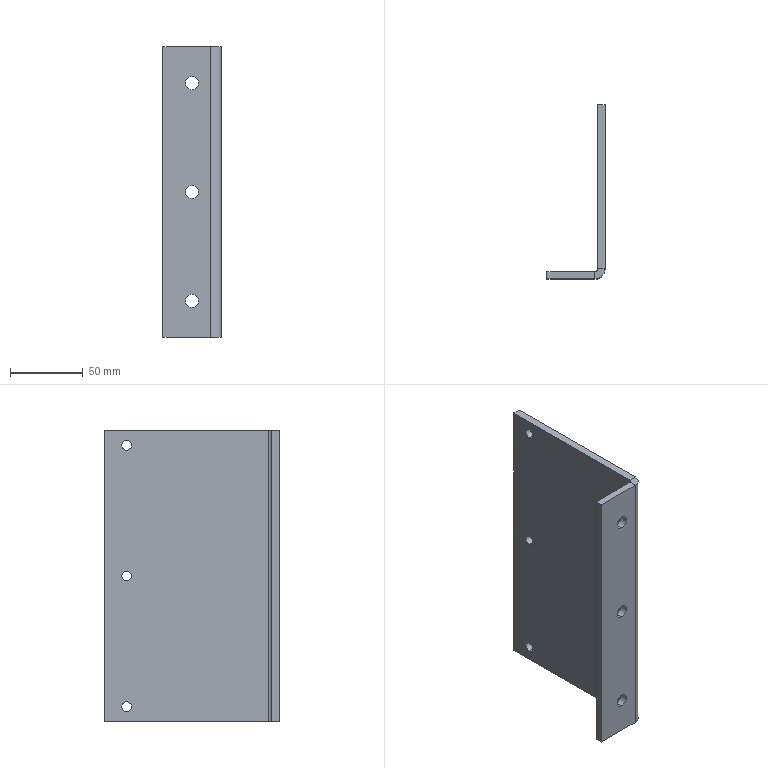Part | SolidWorks | features FlatPattern 1, HoleWzd 1, ICE 1, SMBaseFlange 1, SheetMetal 1 | 1 solid | 26 faces | box 40 x 120 x 200 mm | volume 151570 mm3 | cylinder 14 | plane 12 | commonest cylinder face diameters 6.8 x6 9 x6 4 x1 14 x1
STEP:
#1=CARTESIAN_POINT('',(40.,105.,186.6));
#2=VERTEX_POINT('',#1);
#3=CARTESIAN_POINT('',(40.,105.,193.4));
#4=VERTEX_POINT('',#3);
#5=CARTESIAN_POINT('',(40.,105.,190.));
#6=DIRECTION('',(-1.,0.,0.));
#7=DIRECTION('',(0.,0.,1.));
#8=AXIS2_PLACEMENT_3D('',#5,#6,#7);
#9=CIRCLE('',#8,3.4);
#10=EDGE_CURVE('',#2,#4,#9,.T.);
#11=ORIENTED_EDGE('',*,*,#10,.F.);
#12=CARTESIAN_POINT('',(35.,105.,186.6));
#13=VERTEX_POINT('',#12);
#14=CARTESIAN_POINT('',(35.,105.,186.6));
#15=DIRECTION('',(-1.,0.,0.));
#16=VECTOR('',#15,1000.);
#17=LINE('',#14,#16);
#18=EDGE_CURVE('',#2,#13,#17,.T.);
#19=ORIENTED_EDGE('',*,*,#18,.T.);
#20=CARTESIAN_POINT('',(35.,105.,193.4));
#21=VERTEX_POINT('',#20);
#22=CARTESIAN_POINT('',(35.,105.,190.));
#23=DIRECTION('',(-1.,0.,0.));
#24=DIRECTION('',(0.,0.,1.));
#25=AXIS2_PLACEMENT_3D('',#22,#23,#24);
#26=CIRCLE('',#25,3.4);
#27=EDGE_CURVE('',#13,#21,#26,.T.);
#28=ORIENTED_EDGE('',*,*,#27,.T.);
#29=CARTESIAN_POINT('',(35.,105.,193.4));
#30=DIRECTION('',(-1.,0.,0.));
#31=VECTOR('',#30,1000.);
#32=LINE('',#29,#31);
#33=EDGE_CURVE('',#4,#21,#32,.T.);
#34=ORIENTED_EDGE('',*,*,#33,.F.);
#35=EDGE_LOOP('',(#11,#19,#28,#34));
#36=FACE_OUTER_BOUND('',#35,.T.);
#37=CARTESIAN_POINT('',(35.,105.,190.));
#38=DIRECTION('',(-1.,0.,0.));
#39=DIRECTION('',(0.,0.,1.));
#40=AXIS2_PLACEMENT_3D('',#37,#38,#39);
#41=CYLINDRICAL_SURFACE('',#40,3.4);
#42=ADVANCED_FACE('',(#36),#41,.F.);
#43=CARTESIAN_POINT('',(40.,105.,96.6));
#44=VERTEX_POINT('',#43);
#45=CARTESIAN_POINT('',(40.,105.,103.4));
#46=VERTEX_POINT('',#45);
#47=CARTESIAN_POINT('',(40.,105.,100.));
#48=DIRECTION('',(-1.,0.,0.));
#49=DIRECTION('',(0.,0.,1.));
#50=AXIS2_PLACEMENT_3D('',#47,#48,#49);
#51=CIRCLE('',#50,3.4);
#52=EDGE_CURVE('',#44,#46,#51,.T.);
#53=ORIENTED_EDGE('',*,*,#52,.F.);
#54=CARTESIAN_POINT('',(35.,105.,96.6));
#55=VERTEX_POINT('',#54);
#56=CARTESIAN_POINT('',(35.,105.,96.6));
#57=DIRECTION('',(-1.,0.,0.));
#58=VECTOR('',#57,1000.);
#59=LINE('',#56,#58);
#60=EDGE_CURVE('',#44,#55,#59,.T.);
#61=ORIENTED_EDGE('',*,*,#60,.T.);
#62=CARTESIAN_POINT('',(35.,105.,103.4));
#63=VERTEX_POINT('',#62);
#64=CARTESIAN_POINT('',(35.,105.,100.));
#65=DIRECTION('',(-1.,0.,0.));
#66=DIRECTION('',(0.,0.,1.));
#67=AXIS2_PLACEMENT_3D('',#64,#65,#66);
#68=CIRCLE('',#67,3.4);
#69=EDGE_CURVE('',#55,#63,#68,.T.);
#70=ORIENTED_EDGE('',*,*,#69,.T.);
#71=CARTESIAN_POINT('',(35.,105.,103.4));
#72=DIRECTION('',(-1.,0.,0.));
#73=VECTOR('',#72,1000.);
#74=LINE('',#71,#73);
#75=EDGE_CURVE('',#46,#63,#74,.T.);
#76=ORIENTED_EDGE('',*,*,#75,.F.);
#77=EDGE_LOOP('',(#53,#61,#70,#76));
#78=FACE_OUTER_BOUND('',#77,.T.);
#79=CARTESIAN_POINT('',(35.,105.,100.));
#80=DIRECTION('',(-1.,0.,0.));
#81=DIRECTION('',(0.,0.,1.));
#82=AXIS2_PLACEMENT_3D('',#79,#80,#81);
#83=CYLINDRICAL_SURFACE('',#82,3.4);
#84=ADVANCED_FACE('',(#78),#83,.F.);
#85=CARTESIAN_POINT('',(40.,105.,6.6));
#86=VERTEX_POINT('',#85);
#87=CARTESIAN_POINT('',(40.,105.,13.4));
#88=VERTEX_POINT('',#87);
#89=CARTESIAN_POINT('',(40.,105.,10.));
#90=DIRECTION('',(-1.,0.,0.));
#91=DIRECTION('',(0.,0.,1.));
#92=AXIS2_PLACEMENT_3D('',#89,#90,#91);
#93=CIRCLE('',#92,3.4);
#94=EDGE_CURVE('',#86,#88,#93,.T.);
#95=ORIENTED_EDGE('',*,*,#94,.F.);
#96=CARTESIAN_POINT('',(35.,105.,6.6));
#97=VERTEX_POINT('',#96);
#98=CARTESIAN_POINT('',(35.,105.,6.6));
#99=DIRECTION('',(-1.,0.,0.));
#100=VECTOR('',#99,1000.);
#101=LINE('',#98,#100);
#102=EDGE_CURVE('',#86,#97,#101,.T.);
#103=ORIENTED_EDGE('',*,*,#102,.T.);
#104=CARTESIAN_POINT('',(35.,105.,13.4));
#105=VERTEX_POINT('',#104);
#106=CARTESIAN_POINT('',(35.,105.,10.));
#107=DIRECTION('',(-1.,0.,0.));
#108=DIRECTION('',(0.,0.,1.));
#109=AXIS2_PLACEMENT_3D('',#106,#107,#108);
#110=CIRCLE('',#109,3.4);
#111=EDGE_CURVE('',#97,#105,#110,.T.);
#112=ORIENTED_EDGE('',*,*,#111,.T.);
#113=CARTESIAN_POINT('',(35.,105.,13.4));
#114=DIRECTION('',(-1.,0.,0.));
#115=VECTOR('',#114,1000.);
#116=LINE('',#113,#115);
#117=EDGE_CURVE('',#88,#105,#116,.T.);
#118=ORIENTED_EDGE('',*,*,#117,.F.);
#119=EDGE_LOOP('',(#95,#103,#112,#118));
#120=FACE_OUTER_BOUND('',#119,.T.);
#121=CARTESIAN_POINT('',(35.,105.,10.));
#122=DIRECTION('',(-1.,0.,0.));
#123=DIRECTION('',(0.,0.,1.));
#124=AXIS2_PLACEMENT_3D('',#121,#122,#123);
#125=CYLINDRICAL_SURFACE('',#124,3.4);
#126=ADVANCED_FACE('',(#120),#125,.F.);
#127=CARTESIAN_POINT('',(20.,0.,170.5));
#128=VERTEX_POINT('',#127);
#129=CARTESIAN_POINT('',(20.,0.,179.5));
#130=VERTEX_POINT('',#129);
#131=CARTESIAN_POINT('',(20.,0.,175.));
#132=DIRECTION('',(0.,1.,0.));
#133=DIRECTION('',(0.,0.,1.));
#134=AXIS2_PLACEMENT_3D('',#131,#132,#133);
#135=CIRCLE('',#134,4.5);
#136=EDGE_CURVE('',#128,#130,#135,.T.);
#137=ORIENTED_EDGE('',*,*,#136,.F.);
#138=CARTESIAN_POINT('',(20.,5.,170.5));
#139=VERTEX_POINT('',#138);
#140=CARTESIAN_POINT('',(20.,-5.,170.5));
#141=DIRECTION('',(0.,1.,0.));
#142=VECTOR('',#141,1000.);
#143=LINE('',#140,#142);
#144=EDGE_CURVE('',#128,#139,#143,.T.);
#145=ORIENTED_EDGE('',*,*,#144,.T.);
#146=CARTESIAN_POINT('',(20.,5.,179.5));
#147=VERTEX_POINT('',#146);
#148=CARTESIAN_POINT('',(20.,5.,175.));
#149=DIRECTION('',(0.,1.,0.));
#150=DIRECTION('',(0.,0.,1.));
#151=AXIS2_PLACEMENT_3D('',#148,#149,#150);
#152=CIRCLE('',#151,4.5);
#153=EDGE_CURVE('',#139,#147,#152,.T.);
#154=ORIENTED_EDGE('',*,*,#153,.T.);
#155=CARTESIAN_POINT('',(20.,-5.,179.5));
#156=DIRECTION('',(0.,1.,0.));
#157=VECTOR('',#156,1000.);
#158=LINE('',#155,#157);
#159=EDGE_CURVE('',#130,#147,#158,.T.);
#160=ORIENTED_EDGE('',*,*,#159,.F.);
#161=EDGE_LOOP('',(#137,#145,#154,#160));
#162=FACE_OUTER_BOUND('',#161,.T.);
#163=CARTESIAN_POINT('',(20.,-5.,175.));
#164=DIRECTION('',(0.,1.,0.));
#165=DIRECTION('',(0.,0.,1.));
#166=AXIS2_PLACEMENT_3D('',#163,#164,#165);
#167=CYLINDRICAL_SURFACE('',#166,4.5);
#168=ADVANCED_FACE('',(#162),#167,.F.);
#169=CARTESIAN_POINT('',(20.,0.,95.5));
#170=VERTEX_POINT('',#169);
#171=CARTESIAN_POINT('',(20.,0.,104.5));
#172=VERTEX_POINT('',#171);
#173=CARTESIAN_POINT('',(20.,0.,100.));
#174=DIRECTION('',(0.,1.,0.));
#175=DIRECTION('',(0.,0.,1.));
#176=AXIS2_PLACEMENT_3D('',#173,#174,#175);
#177=CIRCLE('',#176,4.5);
#178=EDGE_CURVE('',#170,#172,#177,.T.);
#179=ORIENTED_EDGE('',*,*,#178,.F.);
#180=CARTESIAN_POINT('',(20.,5.,95.5));
#181=VERTEX_POINT('',#180);
#182=CARTESIAN_POINT('',(20.,-5.,95.5));
#183=DIRECTION('',(0.,1.,0.));
#184=VECTOR('',#183,1000.);
#185=LINE('',#182,#184);
#186=EDGE_CURVE('',#170,#181,#185,.T.);
#187=ORIENTED_EDGE('',*,*,#186,.T.);
#188=CARTESIAN_POINT('',(20.,5.,104.5));
#189=VERTEX_POINT('',#188);
#190=CARTESIAN_POINT('',(20.,5.,100.));
#191=DIRECTION('',(0.,1.,0.));
#192=DIRECTION('',(0.,0.,1.));
#193=AXIS2_PLACEMENT_3D('',#190,#191,#192);
#194=CIRCLE('',#193,4.5);
#195=EDGE_CURVE('',#181,#189,#194,.T.);
#196=ORIENTED_EDGE('',*,*,#195,.T.);
#197=CARTESIAN_POINT('',(20.,-5.,104.5));
#198=DIRECTION('',(0.,1.,0.));
#199=VECTOR('',#198,1000.);
#200=LINE('',#197,#199);
#201=EDGE_CURVE('',#172,#189,#200,.T.);
#202=ORIENTED_EDGE('',*,*,#201,.F.);
#203=EDGE_LOOP('',(#179,#187,#196,#202));
#204=FACE_OUTER_BOUND('',#203,.T.);
#205=CARTESIAN_POINT('',(20.,-5.,100.));
#206=DIRECTION('',(0.,1.,0.));
#207=DIRECTION('',(0.,0.,1.));
#208=AXIS2_PLACEMENT_3D('',#205,#206,#207);
#209=CYLINDRICAL_SURFACE('',#208,4.5);
#210=ADVANCED_FACE('',(#204),#209,.F.);
#211=CARTESIAN_POINT('',(20.,0.,20.5));
#212=VERTEX_POINT('',#211);
#213=CARTESIAN_POINT('',(20.,0.,29.5));
#214=VERTEX_POINT('',#213);
#215=CARTESIAN_POINT('',(20.,0.,25.));
#216=DIRECTION('',(0.,1.,0.));
#217=DIRECTION('',(0.,0.,1.));
#218=AXIS2_PLACEMENT_3D('',#215,#216,#217);
#219=CIRCLE('',#218,4.5);
#220=EDGE_CURVE('',#212,#214,#219,.T.);
#221=ORIENTED_EDGE('',*,*,#220,.F.);
#222=CARTESIAN_POINT('',(20.,5.,20.5));
#223=VERTEX_POINT('',#222);
#224=CARTESIAN_POINT('',(20.,-5.,20.5));
#225=DIRECTION('',(0.,1.,0.));
#226=VECTOR('',#225,1000.);
#227=LINE('',#224,#226);
#228=EDGE_CURVE('',#212,#223,#227,.T.);
#229=ORIENTED_EDGE('',*,*,#228,.T.);
#230=CARTESIAN_POINT('',(20.,5.,29.5));
#231=VERTEX_POINT('',#230);
#232=CARTESIAN_POINT('',(20.,5.,25.));
#233=DIRECTION('',(0.,1.,0.));
#234=DIRECTION('',(0.,0.,1.));
#235=AXIS2_PLACEMENT_3D('',#232,#233,#234);
#236=CIRCLE('',#235,4.5);
#237=EDGE_CURVE('',#223,#231,#236,.T.);
#238=ORIENTED_EDGE('',*,*,#237,.T.);
#239=CARTESIAN_POINT('',(20.,-5.,29.5));
#240=DIRECTION('',(0.,1.,0.));
#241=VECTOR('',#240,1000.);
#242=LINE('',#239,#241);
#243=EDGE_CURVE('',#214,#231,#242,.T.);
#244=ORIENTED_EDGE('',*,*,#243,.F.);
#245=EDGE_LOOP('',(#221,#229,#238,#244));
#246=FACE_OUTER_BOUND('',#245,.T.);
#247=CARTESIAN_POINT('',(20.,-5.,25.));
#248=DIRECTION('',(0.,1.,0.));
#249=DIRECTION('',(0.,0.,1.));
#250=AXIS2_PLACEMENT_3D('',#247,#248,#249);
#251=CYLINDRICAL_SURFACE('',#250,4.5);
#252=ADVANCED_FACE('',(#246),#251,.F.);
#253=CARTESIAN_POINT('',(33.,0.,200.));
#254=VERTEX_POINT('',#253);
#255=CARTESIAN_POINT('',(33.,5.,200.));
#256=VERTEX_POINT('',#255);
#257=CARTESIAN_POINT('',(33.,0.,200.));
#258=DIRECTION('',(0.,1.,0.));
#259=VECTOR('',#258,1000.);
#260=LINE('',#257,#259);
#261=EDGE_CURVE('',#254,#256,#260,.T.);
#262=ORIENTED_EDGE('',*,*,#261,.F.);
#263=CARTESIAN_POINT('',(40.,7.,200.));
#264=VERTEX_POINT('',#263);
#265=CARTESIAN_POINT('',(33.,7.,200.));
#266=DIRECTION('',(0.,0.,1.));
#267=DIRECTION('',(-1.,0.,0.));
#268=AXIS2_PLACEMENT_3D('',#265,#266,#267);
#269=CIRCLE('',#268,7.);
#270=EDGE_CURVE('',#254,#264,#269,.T.);
#271=ORIENTED_EDGE('',*,*,#270,.T.);
#272=CARTESIAN_POINT('',(35.,7.,200.));
#273=VERTEX_POINT('',#272);
#274=CARTESIAN_POINT('',(35.,7.,200.));
#275=DIRECTION('',(1.,0.,0.));
#276=VECTOR('',#275,1000.);
#277=LINE('',#274,#276);
#278=EDGE_CURVE('',#273,#264,#277,.T.);
#279=ORIENTED_EDGE('',*,*,#278,.F.);
#280=CARTESIAN_POINT('',(33.,7.,200.));
#281=DIRECTION('',(0.,0.,1.));
#282=DIRECTION('',(1.,0.,0.));
#283=AXIS2_PLACEMENT_3D('',#280,#281,#282);
#284=CIRCLE('',#283,2.);
#285=EDGE_CURVE('',#256,#273,#284,.T.);
#286=ORIENTED_EDGE('',*,*,#285,.F.);
#287=EDGE_LOOP('',(#262,#271,#279,#286));
#288=FACE_OUTER_BOUND('',#287,.T.);
#289=CARTESIAN_POINT('',(33.,0.,200.));
#290=DIRECTION('',(0.,0.,1.));
#291=DIRECTION('',(1.,0.,0.));
#292=AXIS2_PLACEMENT_3D('',#289,#290,#291);
#293=PLANE('',#292);
#294=ADVANCED_FACE('',(#288),#293,.T.);
#295=CARTESIAN_POINT('',(0.,0.,200.));
#296=VERTEX_POINT('',#295);
#297=CARTESIAN_POINT('',(0.,0.,200.));
#298=DIRECTION('',(1.,0.,0.));
#299=VECTOR('',#298,1000.);
#300=LINE('',#297,#299);
#301=EDGE_CURVE('',#296,#254,#300,.T.);
#302=ORIENTED_EDGE('',*,*,#301,.T.);
#303=ORIENTED_EDGE('',*,*,#261,.T.);
#304=CARTESIAN_POINT('',(0.,5.,200.));
#305=VERTEX_POINT('',#304);
#306=CARTESIAN_POINT('',(0.,5.,200.));
#307=DIRECTION('',(1.,0.,0.));
#308=VECTOR('',#307,1000.);
#309=LINE('',#306,#308);
#310=EDGE_CURVE('',#305,#256,#309,.T.);
#311=ORIENTED_EDGE('',*,*,#310,.F.);
#312=CARTESIAN_POINT('',(0.,0.,200.));
#313=DIRECTION('',(0.,1.,0.));
#314=VECTOR('',#313,1000.);
#315=LINE('',#312,#314);
#316=EDGE_CURVE('',#296,#305,#315,.T.);
#317=ORIENTED_EDGE('',*,*,#316,.F.);
#318=EDGE_LOOP('',(#302,#303,#311,#317));
#319=FACE_OUTER_BOUND('',#318,.T.);
#320=CARTESIAN_POINT('',(35.,7.,200.));
#321=DIRECTION('',(0.,0.,1.));
#322=DIRECTION('',(1.,0.,0.));
#323=AXIS2_PLACEMENT_3D('',#320,#321,#322);
#324=PLANE('',#323);
#325=ADVANCED_FACE('',(#319),#324,.T.);
#326=CARTESIAN_POINT('',(40.,7.,0.));
#327=VERTEX_POINT('',#326);
#328=CARTESIAN_POINT('',(35.,7.,0.));
#329=VERTEX_POINT('',#328);
#330=CARTESIAN_POINT('',(40.,7.,0.));
#331=DIRECTION('',(-1.,0.,0.));
#332=VECTOR('',#331,1000.);
#333=LINE('',#330,#332);
#334=EDGE_CURVE('',#327,#329,#333,.T.);
#335=ORIENTED_EDGE('',*,*,#334,.F.);
#336=CARTESIAN_POINT('',(33.,0.,0.));
#337=VERTEX_POINT('',#336);
#338=CARTESIAN_POINT('',(33.,7.,0.));
#339=DIRECTION('',(0.,0.,1.));
#340=DIRECTION('',(-1.,0.,0.));
#341=AXIS2_PLACEMENT_3D('',#338,#339,#340);
#342=CIRCLE('',#341,7.);
#343=EDGE_CURVE('',#337,#327,#342,.T.);
#344=ORIENTED_EDGE('',*,*,#343,.F.);
#345=CARTESIAN_POINT('',(33.,5.,0.));
#346=VERTEX_POINT('',#345);
#347=CARTESIAN_POINT('',(33.,5.,0.));
#348=DIRECTION('',(0.,-1.,0.));
#349=VECTOR('',#348,1000.);
#350=LINE('',#347,#349);
#351=EDGE_CURVE('',#346,#337,#350,.T.);
#352=ORIENTED_EDGE('',*,*,#351,.F.);
#353=CARTESIAN_POINT('',(33.,7.,0.));
#354=DIRECTION('',(0.,0.,1.));
#355=DIRECTION('',(1.,0.,0.));
#356=AXIS2_PLACEMENT_3D('',#353,#354,#355);
#357=CIRCLE('',#356,2.);
#358=EDGE_CURVE('',#346,#329,#357,.T.);
#359=ORIENTED_EDGE('',*,*,#358,.T.);
#360=EDGE_LOOP('',(#335,#344,#352,#359));
#361=FACE_OUTER_BOUND('',#360,.T.);
#362=CARTESIAN_POINT('',(40.,7.,0.));
#363=DIRECTION('',(0.,0.,-1.));
#364=DIRECTION('',(-1.,0.,0.));
#365=AXIS2_PLACEMENT_3D('',#362,#363,#364);
#366=PLANE('',#365);
#367=ADVANCED_FACE('',(#361),#366,.T.);
#368=CARTESIAN_POINT('',(40.,120.,0.));
#369=VERTEX_POINT('',#368);
#370=CARTESIAN_POINT('',(40.,0.,0.));
#371=DIRECTION('',(0.,1.,0.));
#372=VECTOR('',#371,1000.);
#373=LINE('',#370,#372);
#374=EDGE_CURVE('',#327,#369,#373,.T.);
#375=ORIENTED_EDGE('',*,*,#374,.F.);
#376=ORIENTED_EDGE('',*,*,#334,.T.);
#377=CARTESIAN_POINT('',(35.,120.,0.));
#378=VERTEX_POINT('',#377);
#379=CARTESIAN_POINT('',(35.,0.,0.));
#380=DIRECTION('',(0.,1.,0.));
#381=VECTOR('',#380,1000.);
#382=LINE('',#379,#381);
#383=EDGE_CURVE('',#329,#378,#382,.T.);
#384=ORIENTED_EDGE('',*,*,#383,.T.);
#385=CARTESIAN_POINT('',(35.,120.,0.));
#386=DIRECTION('',(1.,0.,0.));
#387=VECTOR('',#386,1000.);
#388=LINE('',#385,#387);
#389=EDGE_CURVE('',#378,#369,#388,.T.);
#390=ORIENTED_EDGE('',*,*,#389,.T.);
#391=EDGE_LOOP('',(#375,#376,#384,#390));
#392=FACE_OUTER_BOUND('',#391,.T.);
#393=CARTESIAN_POINT('',(33.,5.,0.));
#394=DIRECTION('',(0.,0.,-1.));
#395=DIRECTION('',(-1.,0.,0.));
#396=AXIS2_PLACEMENT_3D('',#393,#394,#395);
#397=PLANE('',#396);
#398=ADVANCED_FACE('',(#392),#397,.T.);
#399=CARTESIAN_POINT('',(40.,105.,190.));
#400=DIRECTION('',(-1.,0.,0.));
#401=DIRECTION('',(0.,0.,1.));
#402=AXIS2_PLACEMENT_3D('',#399,#400,#401);
#403=CIRCLE('',#402,3.4);
#404=EDGE_CURVE('',#4,#2,#403,.T.);
#405=ORIENTED_EDGE('',*,*,#404,.T.);
#406=ORIENTED_EDGE('',*,*,#10,.T.);
#407=EDGE_LOOP('',(#405,#406));
#408=FACE_BOUND('',#407,.T.);
#409=CARTESIAN_POINT('',(40.,105.,100.));
#410=DIRECTION('',(-1.,0.,0.));
#411=DIRECTION('',(0.,0.,1.));
#412=AXIS2_PLACEMENT_3D('',#409,#410,#411);
#413=CIRCLE('',#412,3.4);
#414=EDGE_CURVE('',#46,#44,#413,.T.);
#415=ORIENTED_EDGE('',*,*,#414,.T.);
#416=ORIENTED_EDGE('',*,*,#52,.T.);
#417=EDGE_LOOP('',(#415,#416));
#418=FACE_BOUND('',#417,.T.);
#419=CARTESIAN_POINT('',(40.,105.,10.));
#420=DIRECTION('',(-1.,0.,0.));
#421=DIRECTION('',(0.,0.,1.));
#422=AXIS2_PLACEMENT_3D('',#419,#420,#421);
#423=CIRCLE('',#422,3.4);
#424=EDGE_CURVE('',#88,#86,#423,.T.);
#425=ORIENTED_EDGE('',*,*,#424,.T.);
#426=ORIENTED_EDGE('',*,*,#94,.T.);
#427=EDGE_LOOP('',(#425,#426));
#428=FACE_BOUND('',#427,.T.);
#429=ORIENTED_EDGE('',*,*,#374,.T.);
#430=CARTESIAN_POINT('',(40.,120.,200.));
#431=VERTEX_POINT('',#430);
#432=CARTESIAN_POINT('',(40.,120.,200.));
#433=DIRECTION('',(0.,0.,-1.));
#434=VECTOR('',#433,1000.);
#435=LINE('',#432,#434);
#436=EDGE_CURVE('',#431,#369,#435,.T.);
#437=ORIENTED_EDGE('',*,*,#436,.F.);
#438=CARTESIAN_POINT('',(40.,0.,200.));
#439=DIRECTION('',(0.,1.,0.));
#440=VECTOR('',#439,1000.);
#441=LINE('',#438,#440);
#442=EDGE_CURVE('',#264,#431,#441,.T.);
#443=ORIENTED_EDGE('',*,*,#442,.F.);
#444=CARTESIAN_POINT('',(40.,7.,200.));
#445=DIRECTION('',(0.,0.,-1.));
#446=VECTOR('',#445,1000.);
#447=LINE('',#444,#446);
#448=EDGE_CURVE('',#264,#327,#447,.T.);
#449=ORIENTED_EDGE('',*,*,#448,.T.);
#450=EDGE_LOOP('',(#429,#437,#443,#449));
#451=FACE_OUTER_BOUND('',#450,.T.);
#452=CARTESIAN_POINT('',(40.,0.,200.));
#453=DIRECTION('',(-1.,0.,0.));
#454=DIRECTION('',(0.,0.,1.));
#455=AXIS2_PLACEMENT_3D('',#452,#453,#454);
#456=PLANE('',#455);
#457=ADVANCED_FACE('',(#408,#418,#428,#451),#456,.F.);
#458=ORIENTED_EDGE('',*,*,#389,.F.);
#459=CARTESIAN_POINT('',(35.,120.,200.));
#460=VERTEX_POINT('',#459);
#461=CARTESIAN_POINT('',(35.,120.,200.));
#462=DIRECTION('',(0.,0.,-1.));
#463=VECTOR('',#462,1000.);
#464=LINE('',#461,#463);
#465=EDGE_CURVE('',#460,#378,#464,.T.);
#466=ORIENTED_EDGE('',*,*,#465,.F.);
#467=CARTESIAN_POINT('',(35.,120.,200.));
#468=DIRECTION('',(1.,0.,0.));
#469=VECTOR('',#468,1000.);
#470=LINE('',#467,#469);
#471=EDGE_CURVE('',#460,#431,#470,.T.);
#472=ORIENTED_EDGE('',*,*,#471,.T.);
#473=ORIENTED_EDGE('',*,*,#436,.T.);
#474=EDGE_LOOP('',(#458,#466,#472,#473));
#475=FACE_OUTER_BOUND('',#474,.T.);
#476=CARTESIAN_POINT('',(35.,120.,200.));
#477=DIRECTION('',(0.,1.,0.));
#478=DIRECTION('',(0.,0.,1.));
#479=AXIS2_PLACEMENT_3D('',#476,#477,#478);
#480=PLANE('',#479);
#481=ADVANCED_FACE('',(#475),#480,.T.);
#482=CARTESIAN_POINT('',(35.,105.,190.));
#483=DIRECTION('',(-1.,0.,0.));
#484=DIRECTION('',(0.,0.,1.));
#485=AXIS2_PLACEMENT_3D('',#482,#483,#484);
#486=CIRCLE('',#485,3.4);
#487=EDGE_CURVE('',#21,#13,#486,.T.);
#488=ORIENTED_EDGE('',*,*,#487,.F.);
#489=ORIENTED_EDGE('',*,*,#27,.F.);
#490=EDGE_LOOP('',(#488,#489));
#491=FACE_BOUND('',#490,.T.);
#492=CARTESIAN_POINT('',(35.,105.,100.));
#493=DIRECTION('',(-1.,0.,0.));
#494=DIRECTION('',(0.,0.,1.));
#495=AXIS2_PLACEMENT_3D('',#492,#493,#494);
#496=CIRCLE('',#495,3.4);
#497=EDGE_CURVE('',#63,#55,#496,.T.);
#498=ORIENTED_EDGE('',*,*,#497,.F.);
#499=ORIENTED_EDGE('',*,*,#69,.F.);
#500=EDGE_LOOP('',(#498,#499));
#501=FACE_BOUND('',#500,.T.);
#502=CARTESIAN_POINT('',(35.,105.,10.));
#503=DIRECTION('',(-1.,0.,0.));
#504=DIRECTION('',(0.,0.,1.));
#505=AXIS2_PLACEMENT_3D('',#502,#503,#504);
#506=CIRCLE('',#505,3.4);
#507=EDGE_CURVE('',#105,#97,#506,.T.);
#508=ORIENTED_EDGE('',*,*,#507,.F.);
#509=ORIENTED_EDGE('',*,*,#111,.F.);
#510=EDGE_LOOP('',(#508,#509));
#511=FACE_BOUND('',#510,.T.);
#512=ORIENTED_EDGE('',*,*,#383,.F.);
#513=CARTESIAN_POINT('',(35.,7.,200.));
#514=DIRECTION('',(0.,0.,-1.));
#515=VECTOR('',#514,1000.);
#516=LINE('',#513,#515);
#517=EDGE_CURVE('',#273,#329,#516,.T.);
#518=ORIENTED_EDGE('',*,*,#517,.F.);
#519=CARTESIAN_POINT('',(35.,0.,200.));
#520=DIRECTION('',(0.,1.,0.));
#521=VECTOR('',#520,1000.);
#522=LINE('',#519,#521);
#523=EDGE_CURVE('',#273,#460,#522,.T.);
#524=ORIENTED_EDGE('',*,*,#523,.T.);
#525=ORIENTED_EDGE('',*,*,#465,.T.);
#526=EDGE_LOOP('',(#512,#518,#524,#525));
#527=FACE_OUTER_BOUND('',#526,.T.);
#528=CARTESIAN_POINT('',(35.,0.,200.));
#529=DIRECTION('',(-1.,0.,0.));
#530=DIRECTION('',(0.,0.,1.));
#531=AXIS2_PLACEMENT_3D('',#528,#529,#530);
#532=PLANE('',#531);
#533=ADVANCED_FACE('',(#491,#501,#511,#527),#532,.T.);
#534=ORIENTED_EDGE('',*,*,#358,.F.);
#535=CARTESIAN_POINT('',(33.,5.,200.));
#536=DIRECTION('',(0.,0.,-1.));
#537=VECTOR('',#536,1000.);
#538=LINE('',#535,#537);
#539=EDGE_CURVE('',#256,#346,#538,.T.);
#540=ORIENTED_EDGE('',*,*,#539,.F.);
#541=ORIENTED_EDGE('',*,*,#285,.T.);
#542=ORIENTED_EDGE('',*,*,#517,.T.);
#543=EDGE_LOOP('',(#534,#540,#541,#542));
#544=FACE_OUTER_BOUND('',#543,.T.);
#545=CARTESIAN_POINT('',(33.,7.,200.));
#546=DIRECTION('',(0.,0.,-1.));
#547=DIRECTION('',(-1.,0.,0.));
#548=AXIS2_PLACEMENT_3D('',#545,#546,#547);
#549=CYLINDRICAL_SURFACE('',#548,2.);
#550=ADVANCED_FACE('',(#544),#549,.F.);
#551=CARTESIAN_POINT('',(20.,5.,175.));
#552=DIRECTION('',(0.,1.,0.));
#553=DIRECTION('',(0.,0.,1.));
#554=AXIS2_PLACEMENT_3D('',#551,#552,#553);
#555=CIRCLE('',#554,4.5);
#556=EDGE_CURVE('',#147,#139,#555,.T.);
#557=ORIENTED_EDGE('',*,*,#556,.F.);
#558=ORIENTED_EDGE('',*,*,#153,.F.);
#559=EDGE_LOOP('',(#557,#558));
#560=FACE_BOUND('',#559,.T.);
#561=CARTESIAN_POINT('',(20.,5.,100.));
#562=DIRECTION('',(0.,1.,0.));
#563=DIRECTION('',(0.,0.,1.));
#564=AXIS2_PLACEMENT_3D('',#561,#562,#563);
#565=CIRCLE('',#564,4.5);
#566=EDGE_CURVE('',#189,#181,#565,.T.);
#567=ORIENTED_EDGE('',*,*,#566,.F.);
#568=ORIENTED_EDGE('',*,*,#195,.F.);
#569=EDGE_LOOP('',(#567,#568));
#570=FACE_BOUND('',#569,.T.);
#571=CARTESIAN_POINT('',(20.,5.,25.));
#572=DIRECTION('',(0.,1.,0.));
#573=DIRECTION('',(0.,0.,1.));
#574=AXIS2_PLACEMENT_3D('',#571,#572,#573);
#575=CIRCLE('',#574,4.5);
#576=EDGE_CURVE('',#231,#223,#575,.T.);
#577=ORIENTED_EDGE('',*,*,#576,.F.);
#578=ORIENTED_EDGE('',*,*,#237,.F.);
#579=EDGE_LOOP('',(#577,#578));
#580=FACE_BOUND('',#579,.T.);
#581=CARTESIAN_POINT('',(0.,5.,0.));
#582=VERTEX_POINT('',#581);
#583=CARTESIAN_POINT('',(0.,5.,0.));
#584=DIRECTION('',(1.,0.,0.));
#585=VECTOR('',#584,1000.);
#586=LINE('',#583,#585);
#587=EDGE_CURVE('',#582,#346,#586,.T.);
#588=ORIENTED_EDGE('',*,*,#587,.F.);
#589=CARTESIAN_POINT('',(0.,5.,200.));
#590=DIRECTION('',(0.,0.,-1.));
#591=VECTOR('',#590,1000.);
#592=LINE('',#589,#591);
#593=EDGE_CURVE('',#305,#582,#592,.T.);
#594=ORIENTED_EDGE('',*,*,#593,.F.);
#595=ORIENTED_EDGE('',*,*,#310,.T.);
#596=ORIENTED_EDGE('',*,*,#539,.T.);
#597=EDGE_LOOP('',(#588,#594,#595,#596));
#598=FACE_OUTER_BOUND('',#597,.T.);
#599=CARTESIAN_POINT('',(0.,5.,200.));
#600=DIRECTION('',(0.,1.,0.));
#601=DIRECTION('',(0.,0.,1.));
#602=AXIS2_PLACEMENT_3D('',#599,#600,#601);
#603=PLANE('',#602);
#604=ADVANCED_FACE('',(#560,#570,#580,#598),#603,.T.);
#605=CARTESIAN_POINT('',(0.,0.,0.));
#606=VERTEX_POINT('',#605);
#607=CARTESIAN_POINT('',(0.,0.,0.));
#608=DIRECTION('',(0.,1.,0.));
#609=VECTOR('',#608,1000.);
#610=LINE('',#607,#609);
#611=EDGE_CURVE('',#606,#582,#610,.T.);
#612=ORIENTED_EDGE('',*,*,#611,.F.);
#613=CARTESIAN_POINT('',(0.,0.,200.));
#614=DIRECTION('',(0.,0.,-1.));
#615=VECTOR('',#614,1000.);
#616=LINE('',#613,#615);
#617=EDGE_CURVE('',#296,#606,#616,.T.);
#618=ORIENTED_EDGE('',*,*,#617,.F.);
#619=ORIENTED_EDGE('',*,*,#316,.T.);
#620=ORIENTED_EDGE('',*,*,#593,.T.);
#621=EDGE_LOOP('',(#612,#618,#619,#620));
#622=FACE_OUTER_BOUND('',#621,.T.);
#623=CARTESIAN_POINT('',(0.,0.,200.));
#624=DIRECTION('',(-1.,0.,0.));
#625=DIRECTION('',(0.,0.,1.));
#626=AXIS2_PLACEMENT_3D('',#623,#624,#625);
#627=PLANE('',#626);
#628=ADVANCED_FACE('',(#622),#627,.T.);
#629=CARTESIAN_POINT('',(20.,0.,175.));
#630=DIRECTION('',(0.,1.,0.));
#631=DIRECTION('',(0.,0.,1.));
#632=AXIS2_PLACEMENT_3D('',#629,#630,#631);
#633=CIRCLE('',#632,4.5);
#634=EDGE_CURVE('',#130,#128,#633,.T.);
#635=ORIENTED_EDGE('',*,*,#634,.T.);
#636=ORIENTED_EDGE('',*,*,#136,.T.);
#637=EDGE_LOOP('',(#635,#636));
#638=FACE_BOUND('',#637,.T.);
#639=CARTESIAN_POINT('',(20.,0.,100.));
#640=DIRECTION('',(0.,1.,0.));
#641=DIRECTION('',(0.,0.,1.));
#642=AXIS2_PLACEMENT_3D('',#639,#640,#641);
#643=CIRCLE('',#642,4.5);
#644=EDGE_CURVE('',#172,#170,#643,.T.);
#645=ORIENTED_EDGE('',*,*,#644,.T.);
#646=ORIENTED_EDGE('',*,*,#178,.T.);
#647=EDGE_LOOP('',(#645,#646));
#648=FACE_BOUND('',#647,.T.);
#649=CARTESIAN_POINT('',(20.,0.,25.));
#650=DIRECTION('',(0.,1.,0.));
#651=DIRECTION('',(0.,0.,1.));
#652=AXIS2_PLACEMENT_3D('',#649,#650,#651);
#653=CIRCLE('',#652,4.5);
#654=EDGE_CURVE('',#214,#212,#653,.T.);
#655=ORIENTED_EDGE('',*,*,#654,.T.);
#656=ORIENTED_EDGE('',*,*,#220,.T.);
#657=EDGE_LOOP('',(#655,#656));
#658=FACE_BOUND('',#657,.T.);
#659=CARTESIAN_POINT('',(0.,0.,0.));
#660=DIRECTION('',(1.,0.,0.));
#661=VECTOR('',#660,1000.);
#662=LINE('',#659,#661);
#663=EDGE_CURVE('',#606,#337,#662,.T.);
#664=ORIENTED_EDGE('',*,*,#663,.T.);
#665=CARTESIAN_POINT('',(33.,0.,200.));
#666=DIRECTION('',(0.,0.,-1.));
#667=VECTOR('',#666,1000.);
#668=LINE('',#665,#667);
#669=EDGE_CURVE('',#254,#337,#668,.T.);
#670=ORIENTED_EDGE('',*,*,#669,.F.);
#671=ORIENTED_EDGE('',*,*,#301,.F.);
#672=ORIENTED_EDGE('',*,*,#617,.T.);
#673=EDGE_LOOP('',(#664,#670,#671,#672));
#674=FACE_OUTER_BOUND('',#673,.T.);
#675=CARTESIAN_POINT('',(0.,0.,200.));
#676=DIRECTION('',(0.,1.,0.));
#677=DIRECTION('',(0.,0.,1.));
#678=AXIS2_PLACEMENT_3D('',#675,#676,#677);
#679=PLANE('',#678);
#680=ADVANCED_FACE('',(#638,#648,#658,#674),#679,.F.);
#681=ORIENTED_EDGE('',*,*,#343,.T.);
#682=ORIENTED_EDGE('',*,*,#448,.F.);
#683=ORIENTED_EDGE('',*,*,#270,.F.);
#684=ORIENTED_EDGE('',*,*,#669,.T.);
#685=EDGE_LOOP('',(#681,#682,#683,#684));
#686=FACE_OUTER_BOUND('',#685,.T.);
#687=CARTESIAN_POINT('',(33.,7.,200.));
#688=DIRECTION('',(0.,0.,-1.));
#689=DIRECTION('',(-1.,0.,0.));
#690=AXIS2_PLACEMENT_3D('',#687,#688,#689);
#691=CYLINDRICAL_SURFACE('',#690,7.);
#692=ADVANCED_FACE('',(#686),#691,.T.);
#693=ORIENTED_EDGE('',*,*,#442,.T.);
#694=ORIENTED_EDGE('',*,*,#471,.F.);
#695=ORIENTED_EDGE('',*,*,#523,.F.);
#696=ORIENTED_EDGE('',*,*,#278,.T.);
#697=EDGE_LOOP('',(#693,#694,#695,#696));
#698=FACE_OUTER_BOUND('',#697,.T.);
#699=CARTESIAN_POINT('',(33.,7.,200.));
#700=DIRECTION('',(0.,0.,1.));
#701=DIRECTION('',(1.,0.,0.));
#702=AXIS2_PLACEMENT_3D('',#699,#700,#701);
#703=PLANE('',#702);
#704=ADVANCED_FACE('',(#698),#703,.T.);
#705=ORIENTED_EDGE('',*,*,#587,.T.);
#706=ORIENTED_EDGE('',*,*,#351,.T.);
#707=ORIENTED_EDGE('',*,*,#663,.F.);
#708=ORIENTED_EDGE('',*,*,#611,.T.);
#709=EDGE_LOOP('',(#705,#706,#707,#708));
#710=FACE_OUTER_BOUND('',#709,.T.);
#711=CARTESIAN_POINT('',(33.,7.,0.));
#712=DIRECTION('',(0.,0.,1.));
#713=DIRECTION('',(1.,0.,0.));
#714=AXIS2_PLACEMENT_3D('',#711,#712,#713);
#715=PLANE('',#714);
#716=ADVANCED_FACE('',(#710),#715,.F.);
#717=ORIENTED_EDGE('',*,*,#228,.F.);
#718=ORIENTED_EDGE('',*,*,#654,.F.);
#719=ORIENTED_EDGE('',*,*,#243,.T.);
#720=ORIENTED_EDGE('',*,*,#576,.T.);
#721=EDGE_LOOP('',(#717,#718,#719,#720));
#722=FACE_OUTER_BOUND('',#721,.T.);
#723=CARTESIAN_POINT('',(20.,-5.,25.));
#724=DIRECTION('',(0.,1.,0.));
#725=DIRECTION('',(0.,0.,1.));
#726=AXIS2_PLACEMENT_3D('',#723,#724,#725);
#727=CYLINDRICAL_SURFACE('',#726,4.5);
#728=ADVANCED_FACE('',(#722),#727,.F.);
#729=ORIENTED_EDGE('',*,*,#186,.F.);
#730=ORIENTED_EDGE('',*,*,#644,.F.);
#731=ORIENTED_EDGE('',*,*,#201,.T.);
#732=ORIENTED_EDGE('',*,*,#566,.T.);
#733=EDGE_LOOP('',(#729,#730,#731,#732));
#734=FACE_OUTER_BOUND('',#733,.T.);
#735=CARTESIAN_POINT('',(20.,-5.,100.));
#736=DIRECTION('',(0.,1.,0.));
#737=DIRECTION('',(0.,0.,1.));
#738=AXIS2_PLACEMENT_3D('',#735,#736,#737);
#739=CYLINDRICAL_SURFACE('',#738,4.5);
#740=ADVANCED_FACE('',(#734),#739,.F.);
#741=ORIENTED_EDGE('',*,*,#144,.F.);
#742=ORIENTED_EDGE('',*,*,#634,.F.);
#743=ORIENTED_EDGE('',*,*,#159,.T.);
#744=ORIENTED_EDGE('',*,*,#556,.T.);
#745=EDGE_LOOP('',(#741,#742,#743,#744));
#746=FACE_OUTER_BOUND('',#745,.T.);
#747=CARTESIAN_POINT('',(20.,-5.,175.));
#748=DIRECTION('',(0.,1.,0.));
#749=DIRECTION('',(0.,0.,1.));
#750=AXIS2_PLACEMENT_3D('',#747,#748,#749);
#751=CYLINDRICAL_SURFACE('',#750,4.5);
#752=ADVANCED_FACE('',(#746),#751,.F.);
#753=ORIENTED_EDGE('',*,*,#102,.F.);
#754=ORIENTED_EDGE('',*,*,#424,.F.);
#755=ORIENTED_EDGE('',*,*,#117,.T.);
#756=ORIENTED_EDGE('',*,*,#507,.T.);
#757=EDGE_LOOP('',(#753,#754,#755,#756));
#758=FACE_OUTER_BOUND('',#757,.T.);
#759=CARTESIAN_POINT('',(35.,105.,10.));
#760=DIRECTION('',(-1.,0.,0.));
#761=DIRECTION('',(0.,0.,1.));
#762=AXIS2_PLACEMENT_3D('',#759,#760,#761);
#763=CYLINDRICAL_SURFACE('',#762,3.4);
#764=ADVANCED_FACE('',(#758),#763,.F.);
#765=ORIENTED_EDGE('',*,*,#60,.F.);
#766=ORIENTED_EDGE('',*,*,#414,.F.);
#767=ORIENTED_EDGE('',*,*,#75,.T.);
#768=ORIENTED_EDGE('',*,*,#497,.T.);
#769=EDGE_LOOP('',(#765,#766,#767,#768));
#770=FACE_OUTER_BOUND('',#769,.T.);
#771=CARTESIAN_POINT('',(35.,105.,100.));
#772=DIRECTION('',(-1.,0.,0.));
#773=DIRECTION('',(0.,0.,1.));
#774=AXIS2_PLACEMENT_3D('',#771,#772,#773);
#775=CYLINDRICAL_SURFACE('',#774,3.4);
#776=ADVANCED_FACE('',(#770),#775,.F.);
#777=ORIENTED_EDGE('',*,*,#18,.F.);
#778=ORIENTED_EDGE('',*,*,#404,.F.);
#779=ORIENTED_EDGE('',*,*,#33,.T.);
#780=ORIENTED_EDGE('',*,*,#487,.T.);
#781=EDGE_LOOP('',(#777,#778,#779,#780));
#782=FACE_OUTER_BOUND('',#781,.T.);
#783=CARTESIAN_POINT('',(35.,105.,190.));
#784=DIRECTION('',(-1.,0.,0.));
#785=DIRECTION('',(0.,0.,1.));
#786=AXIS2_PLACEMENT_3D('',#783,#784,#785);
#787=CYLINDRICAL_SURFACE('',#786,3.4);
#788=ADVANCED_FACE('',(#782),#787,.F.);
#789=CLOSED_SHELL('',(#42,#84,#126,#168,#210,#252,#294,#325,#367,#398,#457,#481,#533,#550,#604,#628,#680,#692,#704,#716,#728,#740,#752,#764,#776,#788));
#790=MANIFOLD_SOLID_BREP('',#789);
#791=CARTESIAN_POINT('',(0.,0.,0.));
#792=DIRECTION('',(0.,0.,1.));
#793=DIRECTION('',(1.,0.,0.));
#794=AXIS2_PLACEMENT_3D('',#791,#792,#793);
#795=(LENGTH_UNIT()NAMED_UNIT(*)SI_UNIT(.MILLI.,.METRE.));
#796=UNCERTAINTY_MEASURE_WITH_UNIT(LENGTH_MEASURE(0.00001),#795,'','');
#797=(NAMED_UNIT(*)PLANE_ANGLE_UNIT()SI_UNIT($,.RADIAN.));
#798=(NAMED_UNIT(*)SI_UNIT($,.STERADIAN.)SOLID_ANGLE_UNIT());
#799=(GEOMETRIC_REPRESENTATION_CONTEXT(3)GLOBAL_UNCERTAINTY_ASSIGNED_CONTEXT((#796))GLOBAL_UNIT_ASSIGNED_CONTEXT((#795,#797,#798))REPRESENTATION_CONTEXT('',''));
#800=ADVANCED_BREP_SHAPE_REPRESENTATION('',(#790,#794),#799);